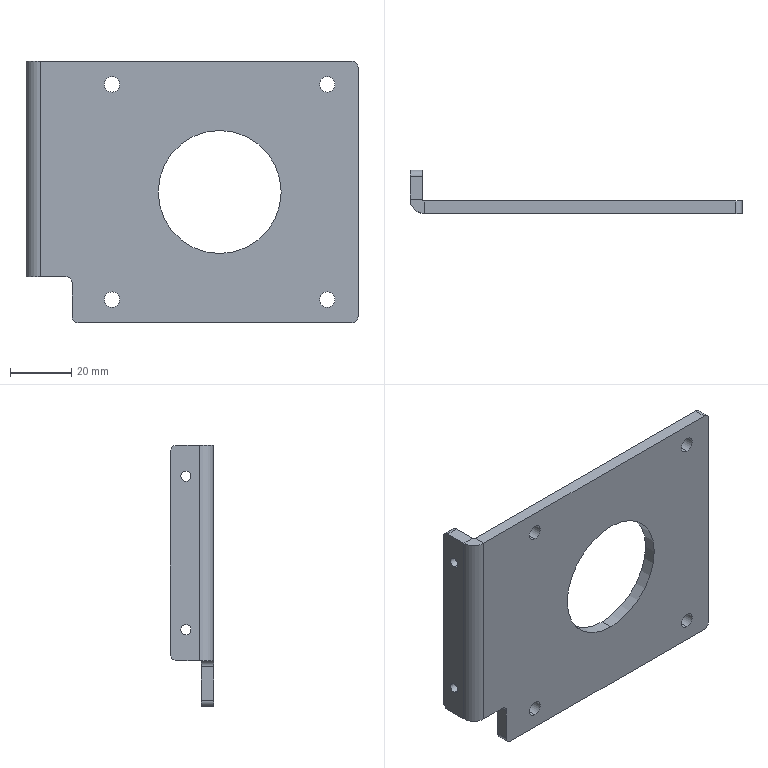Part | STEP file | PN_0001 Tensioning Plate | 1 solid | 36 faces | box 108 x 14 x 85 mm | volume 32885 mm3 | cylinder 22 | plane 14 | commonest cylinder face diameters 5 x8 4 x6 3.3 x4 40 x2 1.2 x1 9.2 x1